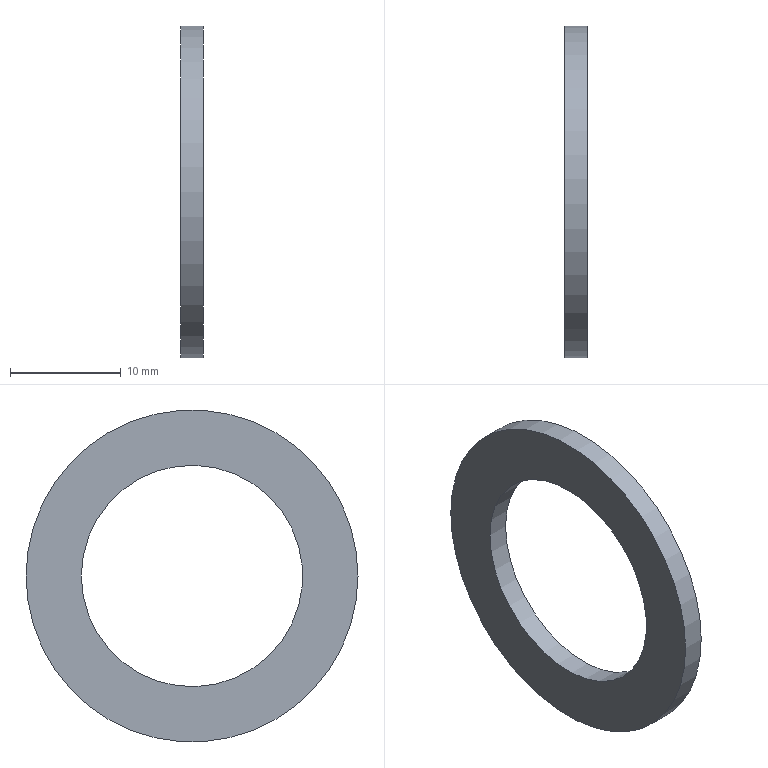Part | NX | features DATUM_CSYS 2, EXTRUDE 1, LINKED_FACE 1, SKETCH 1 | 1 solid | 4 faces | box 2 x 30 x 30 mm | volume 785.398 mm3 | cylinder 2 | plane 2 | commonest cylinder face diameters 20 x1 30 x1
STEP:
#1=CARTESIAN_POINT('',(179.,15.,-133.5));
#2=VERTEX_POINT('',#1);
#3=CARTESIAN_POINT('',(179.,0.,-133.5));
#4=DIRECTION('',(1.,0.,0.));
#5=DIRECTION('',(0.,1.,0.));
#6=AXIS2_PLACEMENT_3D('',#3,#4,#5);
#7=CIRCLE('',#6,15.);
#8=EDGE_CURVE('',#2,#2,#7,.T.);
#9=ORIENTED_EDGE('',*,*,#8,.F.);
#10=EDGE_LOOP('',(#9));
#11=FACE_BOUND('',#10,.T.);
#12=CARTESIAN_POINT('',(177.,15.,-133.5));
#13=VERTEX_POINT('',#12);
#14=CARTESIAN_POINT('',(177.,0.,-133.5));
#15=DIRECTION('',(1.,0.,0.));
#16=DIRECTION('',(0.,1.,0.));
#17=AXIS2_PLACEMENT_3D('',#14,#15,#16);
#18=CIRCLE('',#17,15.);
#19=EDGE_CURVE('',#13,#13,#18,.T.);
#20=ORIENTED_EDGE('',*,*,#19,.T.);
#21=EDGE_LOOP('',(#20));
#22=FACE_BOUND('',#21,.T.);
#23=CARTESIAN_POINT('',(179.,0.,-133.5));
#24=DIRECTION('',(-1.,0.,0.));
#25=DIRECTION('',(0.,-1.,0.));
#26=AXIS2_PLACEMENT_3D('',#23,#24,#25);
#27=CYLINDRICAL_SURFACE('',#26,15.);
#28=ADVANCED_FACE('',(#11,#22),#27,.T.);
#29=CARTESIAN_POINT('',(179.,10.,-133.5));
#30=VERTEX_POINT('',#29);
#31=CARTESIAN_POINT('',(179.,0.,-133.5));
#32=DIRECTION('',(1.,0.,0.));
#33=DIRECTION('',(0.,1.,0.));
#34=AXIS2_PLACEMENT_3D('',#31,#32,#33);
#35=CIRCLE('',#34,10.);
#36=EDGE_CURVE('',#30,#30,#35,.T.);
#37=ORIENTED_EDGE('',*,*,#36,.T.);
#38=EDGE_LOOP('',(#37));
#39=FACE_BOUND('',#38,.T.);
#40=CARTESIAN_POINT('',(177.,10.,-133.5));
#41=VERTEX_POINT('',#40);
#42=CARTESIAN_POINT('',(177.,0.,-133.5));
#43=DIRECTION('',(1.,0.,0.));
#44=DIRECTION('',(0.,1.,0.));
#45=AXIS2_PLACEMENT_3D('',#42,#43,#44);
#46=CIRCLE('',#45,10.);
#47=EDGE_CURVE('',#41,#41,#46,.T.);
#48=ORIENTED_EDGE('',*,*,#47,.F.);
#49=EDGE_LOOP('',(#48));
#50=FACE_BOUND('',#49,.T.);
#51=CARTESIAN_POINT('',(179.,0.,-133.5));
#52=DIRECTION('',(-1.,0.,0.));
#53=DIRECTION('',(0.,-1.,0.));
#54=AXIS2_PLACEMENT_3D('',#51,#52,#53);
#55=CYLINDRICAL_SURFACE('',#54,10.);
#56=ADVANCED_FACE('',(#39,#50),#55,.F.);
#57=ORIENTED_EDGE('',*,*,#8,.T.);
#58=EDGE_LOOP('',(#57));
#59=FACE_BOUND('',#58,.T.);
#60=ORIENTED_EDGE('',*,*,#36,.F.);
#61=EDGE_LOOP('',(#60));
#62=FACE_BOUND('',#61,.T.);
#63=CARTESIAN_POINT('',(179.,0.,-133.5));
#64=DIRECTION('',(1.,0.,0.));
#65=DIRECTION('',(0.,0.,-1.));
#66=AXIS2_PLACEMENT_3D('',#63,#64,#65);
#67=PLANE('',#66);
#68=ADVANCED_FACE('',(#59,#62),#67,.T.);
#69=ORIENTED_EDGE('',*,*,#19,.F.);
#70=EDGE_LOOP('',(#69));
#71=FACE_BOUND('',#70,.T.);
#72=ORIENTED_EDGE('',*,*,#47,.T.);
#73=EDGE_LOOP('',(#72));
#74=FACE_BOUND('',#73,.T.);
#75=CARTESIAN_POINT('',(177.,0.,-133.5));
#76=DIRECTION('',(1.,0.,0.));
#77=DIRECTION('',(0.,0.,-1.));
#78=AXIS2_PLACEMENT_3D('',#75,#76,#77);
#79=PLANE('',#78);
#80=ADVANCED_FACE('',(#71,#74),#79,.F.);
#81=CLOSED_SHELL('',(#28,#56,#68,#80));
#82=MANIFOLD_SOLID_BREP('',#81);
#83=(LENGTH_UNIT()NAMED_UNIT(*)SI_UNIT(.MILLI.,.METRE.));
#84=UNCERTAINTY_MEASURE_WITH_UNIT(LENGTH_MEASURE(0.00001),#83,'','');
#85=(NAMED_UNIT(*)PLANE_ANGLE_UNIT()SI_UNIT($,.RADIAN.));
#86=(NAMED_UNIT(*)SI_UNIT($,.STERADIAN.)SOLID_ANGLE_UNIT());
#87=(GEOMETRIC_REPRESENTATION_CONTEXT(3)GLOBAL_UNCERTAINTY_ASSIGNED_CONTEXT((#84))GLOBAL_UNIT_ASSIGNED_CONTEXT((#83,#85,#86))REPRESENTATION_CONTEXT('',''));
#88=ADVANCED_BREP_SHAPE_REPRESENTATION('',(#82),#87);